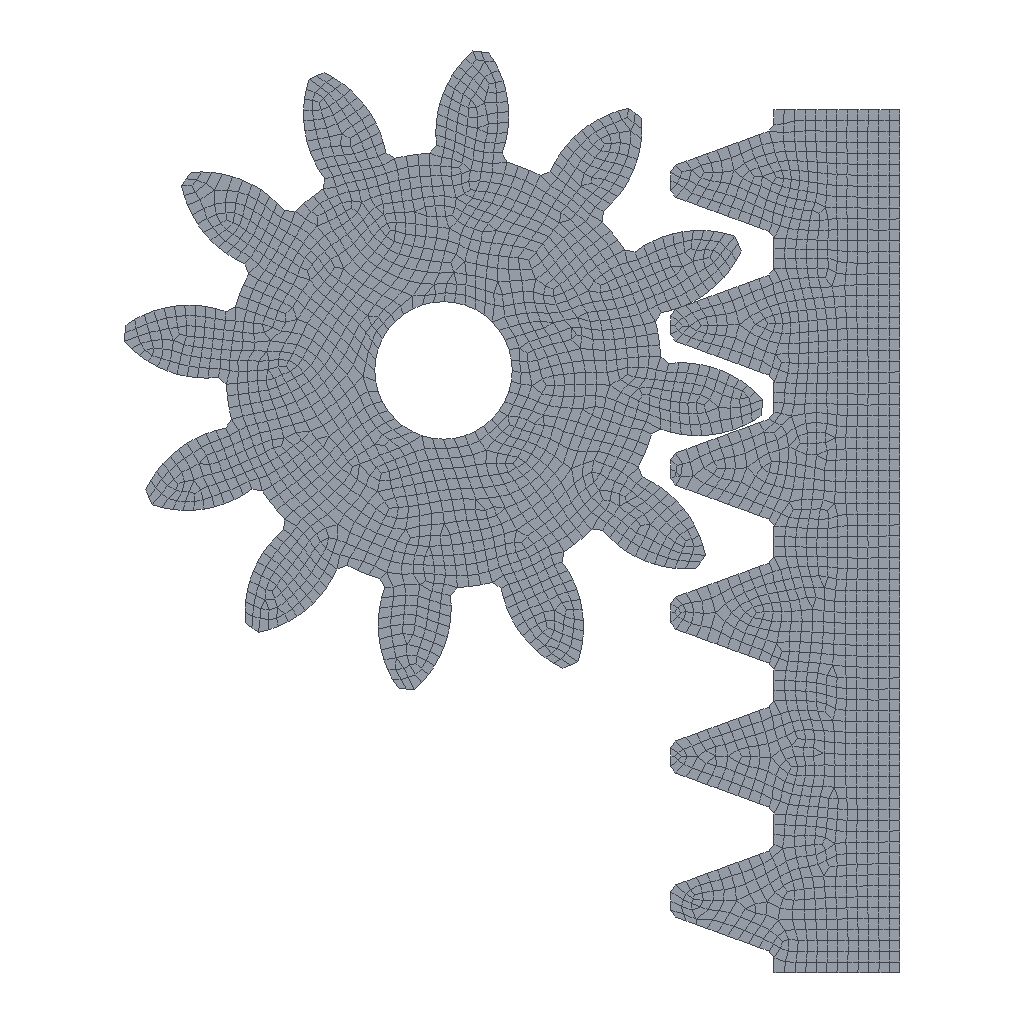Simulation study | ansys workbench
Set-up summary:
category,name,step,type,value,unit,region
solver,ansys_workbench
units,mm-N-s-tonne (MPa),,stated,"/units,MPA"
analysis,LS1,,static
load_step,LS1,LS1,static,nsubst=1; time=1
mesh,nodes,,,10702
mesh,elements,,,3484
element_type,PLANE183,,,3374
element_type,CONTA172,,,69
element_type,TARGE169,,,29
element_type,SURF153,,,12
material,Structural Steel,,E,200000,tonne s^-2 mm^-1
material,Structural Steel,,nu,0.3
material,Structural Steel,,density,7.85e-09,tonne mm^-3
material,Structural Steel,,conductivity,60.5,tonne mm s^-3 C^-1
material,Structural Steel,,specific_heat,4.34e+08,mm^2 s^-2 C^-1
material,Structural Steel,,cte,1.2e-05,C^-1
material,Structural Steel,,permeability,10000
material,Structural Steel,,resistivity,0.00017,ohm mm
load,Define Force Using Surface Effect Elements,LS1,surface-effect pres face 2,11.93,,SURF153 #5
bc,Frictionless Supports X,model,fixed,[dofs=UX],,_FRICSUX
bc,,LS1,fixed,"[dofs=ROTZ,UX,UY n=3]",,node list
contact,No Separation - eg4-FreeParts To eg4-FreeParts[2],,no separation (always),element=CONTA172
contact,contact 2,,bonded (always),element=CONTA172
named_set,_FRICSUX,,node,159
named_set,REMOTEDISPALL,,node,1
Ansys APDL input file, long lists of numbers shortened:
/batch
/config,noeldb,1     ! force off writing results to database
*get,_wallstrt,active,,time,wall
! ANSYS input file written by Workbench version 19.2 RELEASE
! File used for geometry attach:
/title,[REDACTED]
*DIM,_wb_ProjectScratch_dir,string,248
_wb_ProjectScratch_dir(1) = ''
*DIM,_wb_SolverFiles_dir,string,248
_wb_SolverFiles_dir(1) = ''
*DIM,_wb_userfiles_dir,string,248
_wb_userfiles_dir(1) = ''
/com,--- Data in consistent NMM units. See Solving Units in the help system for more information.
/units,MPA
/nopr
/wb,file,start              !  signify a WB generated input file
/prep7
! Turn off shape checking because checks already performed inside WB mesher.
! See help system for more information.
SHPP,OFF,,NOWARN
/nolist
etcon,set             ! allow ANSYS to choose best KEYOP's for 180x elements
/com,*********** Nodes for the whole assembly ***********
nblock,3,,11771
(1i9,3e20.9e3)
        1     9.472639254E+01     9.766173567E+01     0.000000000E+00
! (10700 more lines like these left out)
-1
/com,*********** Nodes for all Remote Points ***********
nblock,3
(1i9,3e20.9e3)
    10702     4.893889228E+01     8.350002494E+01     0.000000000E+00
-1
/wb,elem,start            !  set before creation of elements
/com,*********** Elements for Body 1 "eg4-FreeParts" ***********
et,1,183
keyo,1,3,3
eblock,19,solid,,1399
(19i9)
        1        1        1        1        0        0        0        0        8        0        1      251      250     1200     1200     2029     2031     1200     2032
! (1398 more lines like these left out)
-1
/com,*********** Elements for Body 2 "eg4-FreeParts[2]" ***********
et,2,183
keyo,2,3,3
eblock,19,solid,,1975
(19i9)
        2        2        2        2        0        0        0        0        8        0     1400     6386     6121     5855     5855    10296     9920     5855     9922
! (1974 more lines like these left out)
-1
/wb,elem,end               !  done creating elements
/com,*********** Send User Defined Coordinate System(s) ***********
csys,0
toffst,273.15,  ! Temperature offset from absolute zero
/com,*********** Set Reference Temperature ***********
tref,22.
/wb,mat,start              !  starting to send materials
/com,*********** Send Materials ***********
Temperature = 'TEMP' ! Temperature
MP,DENS,1,7.85e-09,	! tonne mm^-3
MP,ALPX,1,1.2e-05,	! C^-1
MP,C,1,434000000,	! mm^2 s^-2 C^-1
MP,KXX,1,60.5,	! tonne mm s^-3 C^-1
MP,RSVX,1,0.00017,	! ohm mm
MP,EX,1,200000,	! tonne s^-2 mm^-1
MP,NUXY,1,0.3,
MP,MURX,1,10000,
Temperature = 'TEMP' ! Temperature
MP,DENS,2,7.85e-09,	! tonne mm^-3
MP,ALPX,2,1.2e-05,	! C^-1
MP,C,2,434000000,	! mm^2 s^-2 C^-1
MP,KXX,2,60.5,	! tonne mm s^-3 C^-1
MP,RSVX,2,0.00017,	! ohm mm
MP,EX,2,200000,	! tonne s^-2 mm^-1
MP,NUXY,2,0.3,
MP,MURX,2,10000,
/wb,mat,end                !  done sending materials
/com,*********** Send Sheet Properties ***********
r,1,12.
r,2,12.
!************************* Model Summary ********************
!eg4-FreeParts,	Structural Steel,	matid,	1
!eg4-FreeParts[2],	Structural Steel,	matid,	2
!************************* End Model Summary ********************
! get the diagonal of the bounding box. Needed later for other things
*get,_xmin,node,,mnloc,x
*get,_ymin,node,,mnloc,y
*get,_zmin,node,,mnloc,z
*get,_xmax,node,,mxloc,x
*get,_ymax,node,,mxloc,y
*get,_zmax,node,,mxloc,z
_ASMDIAG=(_xmax-_xmin)*(_xmax-_xmin)+(_ymax-_ymin)*(_ymax-_ymin)+(_zmax-_zmin)*(_zmax-_zmin)
_ASMDIAG=SQRT(_ASMDIAG)
/wb,contact,start          !  starting to send contact
/com,*********** Create Contact "No Separation - eg4-FreeParts To eg4-FreeParts[2]" ***********
/com,            Real Constant Set For Above Contact Is 4 & 3
*set,tid,4
*set,cid,3
r,tid
r,cid
et,tid,169
et,cid,172
eblock,10,,,14
(15i9)
     3376        4        4        4        0       11        3     1532
! (13 more lines like these left out)
-1
eblock,10,,,14
(15i9)
     3390        3        3        3        0       11        3     1532
! (13 more lines like these left out)
-1
eblock,10,,,15
(15i9)
     3404        3        4        3        0     4534     4536     6764
! (14 more lines like these left out)
-1
eblock,10,,,15
(15i9)
     3419        4        3        4        0     4534     4536     6764
! (14 more lines like these left out)
-1
keyo,cid,8,2               ! auto create asymmetric contact (from Program Controlled setting)
keyo,cid,10,0              ! adjust contact stiffness each NR iteration (from Program Controlled setting)
keyo,cid,12,4              ! no separation always
keyo,cid,18,1              ! small sliding turned on by application
keyo,cid,2,0               ! augmented Lagrange (from Program Controlled setting)
keyo,cid,4,0               ! on Gauss point (from Program Controlled setting)
keyo,cid,9,1               ! ignore initial gaps/penetration
keyo,cid,7,0               ! No Prediction
rmod,tid,3,10.      ! FKN
rmod,tid,5,0.       ! ICONT
rmod,tid,6,-0.4905 ! PINB
rmod,tid,10,0.      ! CNOF
rmod,tid,12,0.      ! FKT
rmod,tid,36,27      ! WB DSID
rmod,cid,3,10.      ! FKN
rmod,cid,5,0.       ! ICONT
rmod,cid,6,-0.4905 ! PINB
rmod,cid,10,0.      ! CNOF
rmod,cid,12,0.      ! FKT
rmod,cid,36,27      ! WB DSID
nsel,all
esel,all
/wb,contact,end            !  done creating contacts
/golist
/wb,load,start             !  starting to send loads
/com,********* Frictionless Supports X *********
CMBLOCK,_FRICSUX,NODE,      159
(8i10)
       135       147       148       149       150       151       152       153
! (19 more lines like these left out)
cmsel,s,_FRICSUX
d,all,ux,0
nsel,all
/com,*********** Define Force Using Surface Effect Elements ***********
local,12,0,0.,0.,0.,0.,0.,0.
csys,0
et,5,153
keyop,5,3,10   !get plane stress option and thickness from underlying element
eblock,10,,,12
(15i9)
     3434        5        5        5       12      146      145     1821
! (11 more lines like these left out)
-1
esel,s,type,,5
keyop,5,2,1                ! Apply load in local coordinate system
keyop,5,7,1                ! Use original area so load is constant in large deformation
keyop,5,11,2               ! Use real and not project area
esel,all
/com,*********** Create Remote Point "Remote Point" ***********
*set,tid,7
*set,cid,6
et,cid,172
et,tid,169
keyo,tid,2,1               ! Don't fix the pilot node
keyo,tid,4,000111
keyo,cid,12,5              ! Bonded Contact
keyo,cid,4,1               ! Deformable RBE3 style load
keyo,cid,2,2               ! MPC style contact
eblock,10,,,40
(15i9)
     3446        6        6        6        0     4777     4778     7256
! (39 more lines like these left out)
-1
*set,_npilot,10702
_npilot34=_npilot
type,tid
mat ,cid
real,cid
tshape,pilo
en,3486,_npilot
tshape
/com,*********** Construct Remote Displacement ***********
/COM,*** Create a component for all remote displacements ***
CMBLOCK,REMOTEDISPALL,NODE,        1
(8i10)
     10702
/gst,on,on
fini
*get,_numnode,node,0,count
*get,_numelem,elem,0,count
*get, _MAXELEMNUM, elem, 0, NUM, MAX
*get, _MAXNODENUM, node, 0, NUM, MAX
*get, _MAXELEMTYPE, etyp, 0, NUM, MAX
*get, _MAXREALCONST, real, 0, NUM, MAX
/go
/wb,load,end               !  done creating loads
/com,--- Number of total nodes = %_numnode%
/com,--- Number of contact elements = 110
/com,--- Number of spring elements = 0
/com,--- Number of bearing elements = 0
/com,--- Number of solid elements = 3374
/com,--- Number of condensed parts = 0
/com,--- Number of total elements = %_numelem%
*get,_wallbsol,active,,time,wall
/com,****************************************************************************
/com,*************************    SOLUTION       ********************************
/com,****************************************************************************
/solu
antype,0                   ! static analysis
eqsl,sparse,,,,,1
cntr,print,1               ! print out contact info and also make no initial contact an error
dmpoption,emat,no             ! Don't combine emat file for DANSYS
dmpoption,esav,no             ! Don't combine esav file for DANSYS
nldiag,cont,iter           ! print out contact info each equilibrium iteration
rescontrol,,none                 ! Do not keep any restart files
/com,****************************************************
/com,******************* SOLVE FOR LS 1 OF 1 ****************
esel,s,type,,5
nsle
sfe,all,1,pres,1,0.
sfe,all,2,pres,1,11.93
nsel,all
esel,all
d,10702,ux,0.
d,10702,uy,0.
d,10702,rotz,0.
/nopr
/gopr
nsub,1,1,1
time,1.
outres,erase
outres,all,none
outres,nsol,all,
outres,rsol,all
outres,strs,all,
outres,epel,all,
outres,eppl,all,
stabilize,off                   ! Stabilization turned OFF by user
! *********** WB SOLVE COMMAND ***********
! check interactive state
*get,ANSINTER_,active,,int
*if,ANSINTER_,ne,0,then
/eof
*endif
solve
/com *************** Write FE CONNECTORS *********
CEWRITE,file,ce,,INTE
/com,****************************************************
/com,*************** FINISHED SOLVE FOR LS 1 *************
*get,_wallasol,active,,time,wall
/nopr
*get,_numnode,node,0,count
*get,_numelem,elem,0,count
*get, _MAXELEMNUM, elem, 0, NUM, MAX
*get, _MAXNODENUM, node, 0, NUM, MAX,,,INTERNAL
*get, _MAXELEMTYPE, etyp, 0, NUM, MAX
*get, _MAXREALCONST, real, 0, NUM, MAX
/gopr
/post1
xmlo,ENCODING,ISO-8859-1
xmlo,parm
/xml,parm,xml
fini
/gopr
*get,_walldone,active,,time,wall
_preptime=(_wallbsol-_wallstrt)*3600
_solvtime=(_wallasol-_wallbsol)*3600
_posttime=(_walldone-_wallasol)*3600
_totaltim=(_walldone-_wallstrt)*3600
/wb,file,end               ! done with WB generated input
Results summary:
result,analyses[0].index,,,1
result,analyses[0].system,,,SYS
result,analyses[0].deck,,,deck.dat
result,analyses[0].solve_status,,,completed
result,analyses[0].analysis_type,,,static
result,analyses[0].physics,,,mechanical
result,analyses[0].unit_system,,,"NMM: mm, ton, N, s, mV, mA, degC"
result,analyses[0].n_sets,,,1
result,analyses[0].load_steps[0].set,set=1,,1
result,analyses[0].load_steps[0].time_or_freq,set=1,,1
result,analyses[0].load_steps[0].max_displacement_magnitude,set=1,,0.01555
result,analyses[0].load_steps[0].max_von_mises_nodal,set=1,,95.777
result,analyses[0].load_steps[0].reaction_force_sum_xyz[1],set=1,,-1.72446e-07
result,analyses[0].load_steps[0].reaction_force_sum_xyz[2],set=1,,-2500
result,analyses[0].load_steps[0].reaction_force_sum_xyz[3],set=1,,0